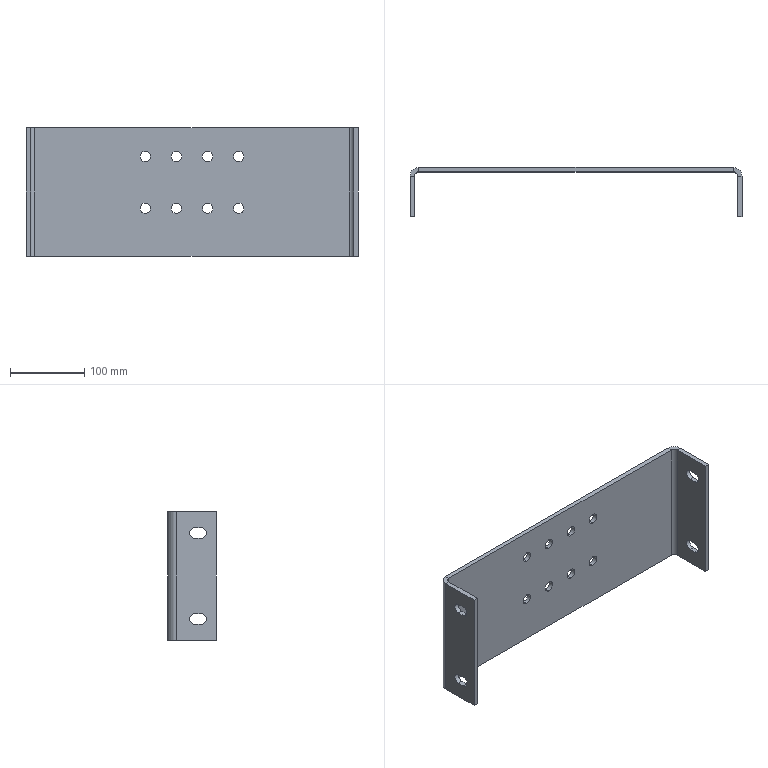Part | STEP file | Anti-jump chain bracket | 1 solid | 54 faces | box 448 x 66 x 174 mm | volume 570819 mm3 | cylinder 28 | plane 26 | commonest cylinder face diameters 14 x24 12 x2 24 x2